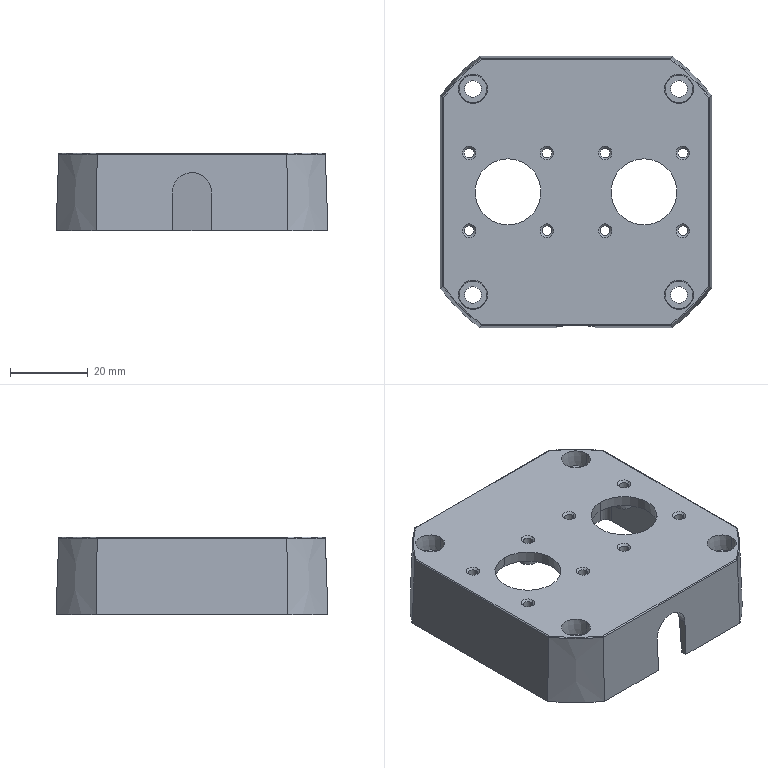Part | SolidWorks | features BaseBody 1 | 1 solid | 126 faces | box 70 x 70 x 20 mm | volume 24252 mm3 | cone 52 | cylinder 37 | plane 33 | spline 4 | commonest cylinder face diameters 2.5 x16 4 x8 4.3 x8 0.5 x4 10 x1